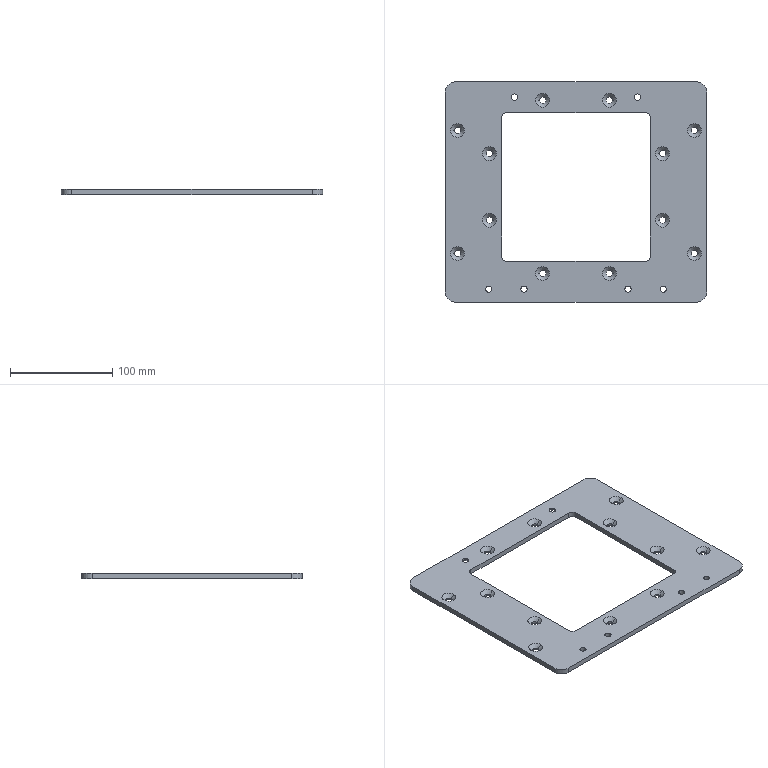NC program | NX | posted with a generic post | part box 255 x 215 x 5 mm
Lines 1056 to 1866 of 7663:
(PLANAR_MILL_COPY_COPY_COPY_COPY , TOOL : D6A45)
N2086 T01 M6
N2088 G54
N2090 G17 G0 G90 X60.866 Y93.85 S9500 M3
N2092 G43 Z30. H1
N2094 Z0.
N2096 G94 G1 Z-1.5 F1250.
N2098 G3 X60. Y94.35 R1.
N2100 X58.15 Y92.5 R1.85
N2102 X60. Y94.35 R-1.85
N2104 X59.134 Y93.85 R1.
N2106 G1 Z0.
N2108 G0 Z30.
N2110 X-59.134
N2112 Z0.
N2114 G1 Z-1.5
N2116 G3 X-60. Y94.35 R1.
N2118 X-61.85 Y92.5 R1.85
N2120 X-60. Y94.35 R-1.85
N2122 X-60.866 Y93.85 R1.
N2124 G1 Z0.
N2126 G0 Z30.
N2128 X0.866 Y75.6
N2130 Z0.
N2132 G1 Z-1.5
N2134 G3 X0. Y76.1 R1.
N2136 G1 X-67.5
N2138 G3 X-71.1 Y72.5 R3.6
N2140 G1 Y-62.5
N2142 G3 X-67.5 Y-66.1 R3.6
N2144 G1 X67.5
N2146 G3 X71.1 Y-62.5 R3.6
N2148 G1 Y72.5
N2150 G3 X67.5 Y76.1 R3.6
N2152 G1 X0.
N2154 G3 X-0.866 Y75.6 R1.
N2156 G1 Z0.
N2158 G0 Z30.
N2160 Y109.4
N2162 Z0.
N2164 G1 Z-1.5
N2166 G3 X0. Y108.9 R1.
N2168 G1 X117.5
N2170 G2 X128.9 Y97.5 R11.4
N2172 G1 Y-97.5
N2174 G2 X117.5 Y-108.9 R11.4
N2176 G1 X-117.5
N2178 G2 X-128.9 Y-97.5 R11.4
N2180 G1 Y97.5
N2182 G2 X-117.5 Y108.9 R11.4
N2184 G1 X0.
N2186 G3 X0.866 Y109.4 R1.
N2188 G1 Z0.
N2190 G0 Z30.
N2192 X-86.116 Y-95.95
N2194 Z0.
N2196 G1 Z-1.5
N2198 G3 X-85.25 Y-96.45 R1.
N2200 X-83.65 Y-94.85 R1.6
N2202 X-85.25 Y-96.45 R-1.6
N2204 X-84.384 Y-95.95 R1.
N2206 G1 Z0.
N2208 G0 Z30.
N2210 X-51.616
N2212 Z0.
N2214 G1 Z-1.5
N2216 G3 X-50.75 Y-96.45 R1.
N2218 X-49.15 Y-94.85 R1.6
N2220 X-50.75 Y-96.45 R-1.6
N2222 X-49.884 Y-95.95 R1.
N2224 G1 Z0.
N2226 G0 Z30.
N2228 X49.884
N2230 Z0.
N2232 G1 Z-1.5
N2234 G3 X50.75 Y-96.45 R1.
N2236 X52.35 Y-94.85 R1.6
N2238 X50.75 Y-96.45 R-1.6
N2240 X51.616 Y-95.95 R1.
N2242 G1 Z0.
N2244 G0 Z30.
N2246 X84.384
N2248 Z0.
N2250 G1 Z-1.5
N2252 G3 X85.25 Y-96.45 R1.
N2254 X86.85 Y-94.85 R1.6
N2256 X85.25 Y-96.45 R-1.6
N2258 X86.116 Y-95.95 R1.
N2260 G1 Z0.
N2262 G0 Z30.
(ZLEVEL_PROFILE_COPY_1_COPY_1 , TOOL : D6A45)
N2264 X90.234 Y-29.265
N2266 Z1.5
N2268 G1 X90.456 Y-28.391 Z1.453 F1000.
N2270 X90.493 Y-28.098 Z1.437
N2272 Y-26.897 Z1.374
N2274 X90.106 Y-25.296 Z1.288
N2276 X89.3 Y-23.86 Z1.202
N2278 X88.136 Y-22.696 Z1.115
N2280 X86.699 Y-21.891 Z1.029
N2282 X85.098 Y-21.505 Z0.943
N2284 X83.453 Y-21.568 Z0.856
N2286 X82.297 Y-21.894 Z0.794
N2288 X80.879 Y-22.687 Z0.708
N2290 X79.725 Y-23.831 Z0.623
N2292 X78.918 Y-25.241 Z0.538
N2294 X78.518 Y-26.816 Z0.453
N2296 X78.554 Y-28.441 Z0.368
N2298 X79.022 Y-29.996 Z0.283
N2300 X79.89 Y-31.37 Z0.197
N2302 X80.75 Y-32.208 Z0.135
N2304 X82.146 Y-33.04 Z0.049
N2306 X83.714 Y-33.468 Z-0.036
N2308 X85.339 Y-33.461 Z-0.121
N2310 X86.903 Y-33.02 Z-0.206
N2312 X88.292 Y-32.177 Z-0.291
N2314 X89.405 Y-30.993 Z-0.376
N2316 X90.161 Y-29.554 Z-0.462
N2318 X90.456 Y-28.391 Z-0.524
N2320 X90.493 Y-28.098 Z-0.54
N2322 Y-27.497 Z-0.571
N2324 G3 X84.501 Y-21.506 R5.992 F1500.
N2326 X90.493 Y-27.497 R-5.992
N2328 G1 X90.44 Y-26.948 Z-0.58
N2330 X90.382 Y-26.4 Z-0.589
N2332 X90.112 Y-25.492 Z-0.604
N2334 X90.061 Y-25.346 Z-0.607
N2336 X89.788 Y-24.792 Z-0.616
N2338 X89.556 Y-24.373 Z-0.624
N2340 X89.203 Y-23.898 Z-0.634
N2342 X88.883 Y-23.511 Z-0.642
N2344 X88.451 Y-23.11 Z-0.651
N2346 X88.066 Y-22.789 Z-0.659
N2348 X87.568 Y-22.473 Z-0.668
N2350 X87.133 Y-22.231 Z-0.676
N2352 X86.584 Y-22.011 Z-0.686
N2354 X86.117 Y-21.855 Z-0.694
N2356 X85.536 Y-21.738 Z-0.703
N2358 X85.052 Y-21.671 Z-0.711
N2360 X84.462 Y-21.663 Z-0.72
N2362 X83.975 Y-21.686 Z-0.728
N2364 X83.391 Y-21.787 Z-0.738
N2366 X82.922 Y-21.897 Z-0.745
N2368 X82.354 Y-22.11 Z-0.755
N2370 X81.898 Y-22.313 Z-0.763
N2372 X81.383 Y-22.627 Z-0.772
N2374 X80.974 Y-22.912 Z-0.78
N2376 X80.18 Y-23.671 Z-0.798
N2378 X80.106 Y-23.766 Z-0.8
N2380 X79.55 Y-24.568 Z-0.816
N2382 X79.307 Y-25.068 Z-0.824
N2384 X79.101 Y-25.563 Z-0.833
N2386 X78.943 Y-26.143 Z-0.843
N2388 X78.848 Y-26.623 Z-0.85
N2390 X78.798 Y-27.21 Z-0.86
N2392 X78.807 Y-27.707 Z-0.868
N2394 X78.848 Y-28.133 Z-0.874
N2396 X78.888 Y-28.492 Z-0.88
N2398 X78.966 Y-28.777 Z-0.885
N2400 X79.135 Y-29.289 Z-0.894
N2402 X79.324 Y-29.795 Z-0.902
N2404 X79.586 Y-30.297 Z-0.911
N2406 X79.867 Y-30.723 Z-0.919
N2408 X80.124 Y-31.049 Z-0.926
N2410 X80.348 Y-31.33 Z-0.932
N2412 X80.573 Y-31.529 Z-0.936
N2414 X80.986 Y-31.868 Z-0.945
N2416 X81.417 Y-32.185 Z-0.954
N2418 X81.746 Y-32.376 Z-0.96
N2420 X82.055 Y-32.553 Z-0.965
N2422 X82.366 Y-32.668 Z-0.971
N2424 X82.871 Y-32.832 Z-0.979
N2426 X83.387 Y-32.961 Z-0.988
N2428 X83.494 Y-32.979 Z-0.989
N2430 X83.966 Y-33.037 Z-0.997
N2432 X84.441 Y-33.056 Z-1.004
N2434 X85.051 Y-33.038 Z-1.014
N2436 X85.197 Y-33.01 Z-1.017
N2438 X85.491 Y-32.95 Z-1.021
N2440 X86.001 Y-32.822 Z-1.03
N2442 X86.499 Y-32.647 Z-1.038
N2444 X86.866 Y-32.491 Z-1.044
N2446 X87.049 Y-32.409 Z-1.048
N2448 X87.428 Y-32.162 Z-1.055
N2450 X87.855 Y-31.859 Z-1.063
N2452 X88.246 Y-31.511 Z-1.072
N2454 X88.538 Y-31.225 Z-1.078
N2456 X88.672 Y-31.071 Z-1.081
N2458 X88.924 Y-30.719 Z-1.088
N2460 X89.206 Y-30.283 Z-1.096
N2462 X89.438 Y-29.817 Z-1.105
N2464 X89.633 Y-29.336 Z-1.113
N2466 X89.772 Y-28.836 Z-1.121
N2468 X89.843 Y-28.506 Z-1.127
N2470 X89.887 Y-28.171 Z-1.132
N2472 X89.906 Y-27.834 Z-1.137
N2474 X89.917 Y-27.497 Z-1.143
N2476 X89.88 Y-27.034 Z-1.151
N2478 X89.843 Y-26.571 Z-1.159
N2480 X89.725 Y-26.16 Z-1.167
N2482 X89.584 Y-25.681 Z-1.176
N2484 X89.307 Y-25.106 Z-1.187
N2486 X89.086 Y-24.668 Z-1.196
N2488 X88.737 Y-24.23 Z-1.206
N2490 X88.378 Y-23.795 Z-1.216
N2492 X87.947 Y-23.429 Z-1.226
N2494 X87.507 Y-23.092 Z-1.235
N2496 X86.992 Y-22.799 Z-1.246
N2498 X86.516 Y-22.585 Z-1.255
N2500 X85.916 Y-22.379 Z-1.266
N2502 X85.447 Y-22.295 Z-1.275
N2504 X84.899 Y-22.229 Z-1.285
N2506 X84.345 Z-1.294
N2508 X83.858 Y-22.261 Z-1.303
N2510 X83.558 Y-22.327 Z-1.308
N2512 X83.257 Y-22.391 Z-1.314
N2514 X82.648 Y-22.606 Z-1.325
N2516 X82.228 Y-22.772 Z-1.333
N2518 X81.72 Y-23.09 Z-1.344
N2520 X81.301 Y-23.354 Z-1.353
N2522 X80.529 Y-24.126 Z-1.372
N2524 X80.23 Y-24.571 Z-1.382
N2526 X79.938 Y-25.037 Z-1.391
N2528 X79.715 Y-25.551 Z-1.401
N2530 X79.545 Y-26.044 Z-1.41
N2532 X79.407 Y-26.645 Z-1.421
N2534 X79.364 Y-27.106 Z-1.43
N2536 X79.38 Y-27.741 Z-1.441
N2538 X79.415 Y-28.179 Z-1.449
N2540 X79.552 Y-28.748 Z-1.459
N2542 X79.681 Y-29.216 Z-1.468
N2544 X80.151 Y-30.175 Z-1.486
N2546 X80.3 Y-30.363 Z-1.491
N2548 X80.445 Y-30.555 Z-1.495
N2550 X80.819 Y-31.004 Z-1.505
N2552 X81.24 Y-31.35 Z-1.515
N2554 X81.643 Y-31.671 Z-1.524
N2556 X82.115 Y-31.93 Z-1.534
N2558 X82.582 Y-32.152 Z-1.543
N2560 X83.111 Y-32.326 Z-1.553
N2562 X83.595 Y-32.429 Z-1.561
N2564 X84.15 Y-32.489 Z-1.571
N2566 X84.566 Y-32.495 Z-1.579
N2568 X85.127 Y-32.441 Z-1.589
N2570 X85.528 Y-32.372 Z-1.596
N2572 X86.049 Y-32.214 Z-1.605
N2574 X86.445 Y-32.066 Z-1.613
N2576 X86.912 Y-31.815 Z-1.622
N2578 X87.283 Y-31.591 Z-1.63
N2580 X87.68 Y-31.26 Z-1.639
N2582 X88.012 Y-30.964 Z-1.647
N2584 X88.325 Y-30.572 Z-1.656
N2586 X88.604 Y-30.211 Z-1.664
N2588 X88.826 Y-29.778 Z-1.672
N2590 X89.039 Y-29.361 Z-1.681
N2592 X89.304 Y-28.445 Z-1.698
N2594 X89.327 Y-27.972 Z-1.706
N2596 X89.349 Y-27.498 Z-1.714
N2598 X89.295 Y-26.856 Z-1.727
N2600 X89.221 Y-26.483 Z-1.735
N2602 X89.106 Y-26.091 Z-1.743
N2604 X89.006 Y-25.766 Z-1.749
N2606 X88.885 Y-25.523 Z-1.755
N2608 X88.633 Y-25.083 Z-1.765
N2610 X88.353 Y-24.661 Z-1.775
N2612 X88.123 Y-24.376 Z-1.782
N2614 X88.005 Y-24.236 Z-1.786
N2616 X87.657 Y-23.93 Z-1.795
N2618 X87.144 Y-23.55 Z-1.808
N2620 X86.829 Y-23.362 Z-1.815
N2622 X86.283 Y-23.117 Z-1.827
N2624 X85.904 Y-22.979 Z-1.835
N2626 X85.357 Y-22.868 Z-1.846
N2628 X84.922 Y-22.801 Z-1.855
N2630 X84.438 Y-22.808 Z-1.865
N2632 X83.928 Y-22.837 Z-1.875
N2634 X83.222 Y-22.992 Z-1.889
N2636 X82.98 Y-23.083 Z-1.894
N2638 X82.539 Y-23.289 Z-1.904
N2640 X82.107 Y-23.516 Z-1.914
N2642 X81.679 Y-23.804 Z-1.924
N2644 X81.565 Y-23.905 Z-1.927
N2646 X81.345 Y-24.115 Z-1.933
N2648 X80.922 Y-24.58 Z-1.946
N2650 X80.725 Y-24.856 Z-1.952
N2652 X80.43 Y-25.361 Z-1.964
N2654 X80.271 Y-25.704 Z-1.972
N2656 X80.093 Y-26.255 Z-1.983
N2658 X79.996 Y-26.624 Z-1.991
N2660 X79.944 Y-27.146 Z-2.001
N2662 X79.928 Y-27.579 Z-2.01
N2664 X79.992 Y-28.073 Z-2.02
N2666 X80.069 Y-28.522 Z-2.029
N2668 X80.228 Y-28.999 Z-2.039
N2670 X80.397 Y-29.412 Z-2.048
N2672 X80.635 Y-29.831 Z-2.057
N2674 X80.899 Y-30.212 Z-2.067
N2676 X81.365 Y-30.727 Z-2.081
N2678 X81.465 Y-30.802 Z-2.083
N2680 X81.551 Y-30.89 Z-2.085
N2682 X81.946 Y-31.174 Z-2.095
N2684 X82.327 Y-31.418 Z-2.104
N2686 X82.788 Y-31.61 Z-2.114
N2688 X83.193 Y-31.77 Z-2.123
N2690 X83.662 Y-31.855 Z-2.132
N2692 X84.111 Y-31.932 Z-2.141
N2694 X84.577 Y-31.919 Z-2.151
N2696 X85.038 Y-31.898 Z-2.16
N2698 X85.501 Y-31.793 Z-2.169
N2700 X85.935 Y-31.674 Z-2.178
N2702 X86.381 Y-31.477 Z-2.188
N2704 X86.763 Y-31.27 Z-2.197
N2706 X87.185 Y-30.98 Z-2.207
N2708 X87.486 Y-30.705 Z-2.215
N2710 X87.862 Y-30.289 Z-2.226
N2712 X88.074 Y-30.005 Z-2.233
N2714 X88.326 Y-29.574 Z-2.243
N2716 X88.501 Y-29.201 Z-2.251
N2718 X88.605 Y-28.878 Z-2.258
N2720 X88.706 Y-28.555 Z-2.265
N2722 X88.75 Y-28.365 Z-2.268
N2724 X88.794 Y-27.932 Z-2.277
N2726 X88.817 Y-27.498 Z-2.286
N2728 X88.813 Y-27.393 Z-2.288
N2730 X88.808 Y-27.289 Z-2.29
N2732 X88.753 Y-26.784 Z-2.302
N2734 X88.684 Y-26.513 Z-2.308
N2736 X88.559 Y-26.105 Z-2.317
N2738 X88.491 Y-25.903 Z-2.322
N2740 X88.325 Y-25.593 Z-2.33
N2742 X87.967 Y-25.018 Z-2.345
N2744 X87.777 Y-24.777 Z-2.352
N2746 X87.355 Y-24.359 Z-2.365
N2748 X87.059 Y-24.111 Z-2.374
N2750 X86.593 Y-23.825 Z-2.386
N2752 X86.208 Y-23.634 Z-2.396
N2754 X85.705 Y-23.453 Z-2.408
N2756 X85.564 Y-23.415 Z-2.411
N2758 X85.274 Y-23.369 Z-2.417
N2760 X84.609 Y-23.309 Z-2.432
N2762 X84.309 Y-23.317 Z-2.439
N2764 X83.725 Y-23.4 Z-2.452
N2766 X83.361 Y-23.485 Z-2.461
N2768 X82.925 Y-23.653 Z-2.471
N2770 X82.476 Y-23.871 Z-2.482
N2772 X82.358 Y-23.942 Z-2.485
N2774 X82.246 Y-24.022 Z-2.488
N2776 X81.956 Y-24.209 Z-2.496
N2778 X81.71 Y-24.453 Z-2.504
N2780 X81.254 Y-24.962 Z-2.519
N2782 X81.095 Y-25.187 Z-2.525
N2784 X80.817 Y-25.693 Z-2.538
N2786 X80.667 Y-26.039 Z-2.546
N2788 X80.521 Y-26.56 Z-2.559
N2790 X80.451 Y-26.965 Z-2.568
N2792 X80.42 Y-27.32 Z-2.576
N2794 X80.41 Y-27.497 Z-2.58
N2796 X80.457 Y-27.911 Z-2.589
N2798 X80.58 Y-28.521 Z-2.603
N2800 X80.675 Y-28.828 Z-2.61
N2802 X80.903 Y-29.323 Z-2.622
N2804 X81.099 Y-29.666 Z-2.631
N2806 X81.415 Y-30.078 Z-2.643
N2808 X81.704 Y-30.378 Z-2.652
N2810 X82.058 Y-30.682 Z-2.662
N2812 X82.454 Y-30.929 Z-2.673
N2814 X82.679 Y-31.055 Z-2.678
N2816 X83.046 Y-31.203 Z-2.687
N2818 X83.304 Y-31.298 Z-2.693
N2820 X83.817 Y-31.404 Z-2.705
N2822 X84.214 Y-31.454 Z-2.714
N2824 X84.717 Y-31.445 Z-2.725
N2826 X85.132 Y-31.393 Z-2.735
N2828 X85.469 Y-31.317 Z-2.742
N2830 X85.638 Y-31.277 Z-2.746
N2832 X86.006 Y-31.125 Z-2.755
N2834 X86.526 Y-30.847 Z-2.768
N2836 X86.795 Y-30.67 Z-2.775
N2838 X87.18 Y-30.328 Z-2.787
N2840 X87.451 Y-30.043 Z-2.796
N2842 X87.744 Y-29.637 Z-2.807
N2844 X87.941 Y-29.285 Z-2.816
N2846 X88.13 Y-28.866 Z-2.826
N2848 X88.17 Y-28.725 Z-2.829
N2850 X88.243 Y-28.439 Z-2.836
N2852 X88.286 Y-28.206 Z-2.841
N2854 X88.322 Y-27.971 Z-2.847
N2856 X88.342 Y-27.498 Z-2.857
N2858 X88.336 Y-27.382 Z-2.86
N2860 X88.329 Y-27.267 Z-2.863
N2862 X88.29 Y-26.92 Z-2.872
N2864 X88.261 Y-26.748 Z-2.876
N2866 X88.229 Y-26.645 Z-2.879
N2868 X88.165 Y-26.438 Z-2.885
N2870 X88.045 Y-26.074 Z-2.894
N2872 X87.907 Y-25.813 Z-2.902
N2874 X87.803 Y-25.631 Z-2.907
N2876 X87.463 Y-25.144 Z-2.922
N2878 X87.274 Y-24.927 Z-2.929
N2880 X86.988 Y-24.666 Z-2.939
N2882 X86.588 Y-24.38 Z-2.952
N2884 X86.353 Y-24.243 Z-2.959
N2886 X86.086 Y-24.106 Z-2.966
N2888 X85.805 Y-24.001 Z-2.974
N2890 X85.274 Y-23.848 Z-2.988
N2892 X84.961 Y-23.801 Z-2.996
N2894 X84.579 Y-23.756 Z-3.006
N2896 X84.29 Y-23.769 Z-3.013
N2898 X84.094 Y-23.79 Z-3.018
N2900 X83.568 Y-23.9 Z-3.031
N2902 X83.256 Y-24.005 Z-3.04
N2904 X82.794 Y-24.22 Z-3.053
N2906 X82.494 Y-24.404 Z-3.061
N2908 X82.1 Y-24.715 Z-3.074
N2910 X81.85 Y-24.966 Z-3.083
N2912 X81.541 Y-25.356 Z-3.096
N2914 X81.355 Y-25.656 Z-3.105
N2916 X81.146 Y-26.105 Z-3.117
N2918 X81.035 Y-26.437 Z-3.126
N2920 X80.935 Y-26.919 Z-3.138
N2922 X80.905 Y-27.266 Z-3.147
N2924 X80.919 Y-27.755 Z-3.16
N2926 X80.968 Y-28.097 Z-3.168
N2928 X81.094 Y-28.567 Z-3.181
N2930 X81.22 Y-28.887 Z-3.189
N2932 X81.449 Y-29.312 Z-3.202
N2934 X81.645 Y-29.593 Z-3.21
N2936 X81.964 Y-29.952 Z-3.222
N2938 X82.217 Y-30.178 Z-3.231
N2940 X82.606 Y-30.451 Z-3.243
N2942 X82.905 Y-30.614 Z-3.252
N2944 X83.333 Y-30.786 Z-3.263
N2946 X83.652 Y-30.873 Z-3.272
N2948 X84.107 Y-30.944 Z-3.283
N2950 X84.433 Y-30.958 Z-3.292
N2952 X84.89 Y-30.925 Z-3.303
N2954 X85.209 Y-30.865 Z-3.312
N2956 X85.645 Y-30.73 Z-3.323
N2958 X85.94 Y-30.601 Z-3.331
N2960 X86.332 Y-30.373 Z-3.343
N2962 X86.589 Y-30.181 Z-3.351
N2964 X86.872 Y-29.921 Z-3.361
N2966 X87.124 Y-29.629 Z-3.371
N2968 X87.198 Y-29.529 Z-3.374
N2970 X87.269 Y-29.427 Z-3.377
N2972 X87.403 Y-29.206 Z-3.383
N2974 X87.519 Y-28.975 Z-3.39
N2976 X87.68 Y-28.548 Z-3.402
N2978 X87.755 Y-28.252 Z-3.409
N2980 X87.81 Y-27.878 Z-3.419
N2982 X87.821 Y-27.499 Z-3.429
N2984 X87.817 Y-27.398 Z-3.432
N2986 X87.809 Y-27.299 Z-3.435
N2988 X87.72 Y-26.781 Z-3.45
N2990 X87.635 Y-26.5 Z-3.459
N2992 X87.44 Y-26.055 Z-3.474
N2994 X87.272 Y-25.773 Z-3.484
N2996 X86.983 Y-25.4 Z-3.498
N2998 X86.745 Y-25.163 Z-3.508
N3000 X86.371 Y-24.872 Z-3.522
N3002 X86.09 Y-24.705 Z-3.532
N3004 X85.649 Y-24.522 Z-3.546
N3006 X85.33 Y-24.419 Z-3.556
N3008 X84.892 Y-24.353 Z-3.57
N3010 X84.53 Y-24.334 Z-3.581
N3012 X84.085 Y-24.38 Z-3.594
N3014 X83.74 Y-24.453 Z-3.605
N3016 X83.322 Y-24.615 Z-3.618
N3018 X83.011 Y-24.763 Z-3.629
N3020 X82.657 Y-25.005 Z-3.642
N3022 X82.388 Y-25.243 Z-3.653
N3024 X82.101 Y-25.585 Z-3.666
N3026 X81.91 Y-25.859 Z-3.676
N3028 X81.721 Y-26.253 Z-3.689
N3030 X81.603 Y-26.57 Z-3.699
N3032 X81.538 Y-26.829 Z-3.707
N3034 X81.514 Y-26.961 Z-3.712
N3036 X81.505 Y-27.083 Z-3.715
N3038 X81.49 Y-27.329 Z-3.723
N3040 X81.513 Y-27.74 Z-3.735
N3042 X81.542 Y-27.992 Z-3.743
N3044 X81.631 Y-28.345 Z-3.754
N3046 X81.741 Y-28.623 Z-3.763
N3048 X81.895 Y-28.92 Z-3.773
N3050 X82.079 Y-29.185 Z-3.783
N3052 X82.43 Y-29.592 Z-3.799
N3054 X82.559 Y-29.705 Z-3.804
N3056 X82.917 Y-29.959 Z-3.817
N3058 X83.15 Y-30.085 Z-3.825
N3060 X83.523 Y-30.223 Z-3.837
N3062 X83.811 Y-30.308 Z-3.846
N3064 X84.199 Y-30.364 Z-3.858
N3066 X84.501 Y-30.375 Z-3.867
N3068 X84.88 Y-30.334 Z-3.879
N3070 X85.181 Y-30.271 Z-3.888
N3072 X85.546 Y-30.127 Z-3.9
N3074 X85.813 Y-30.013 Z-3.909
N3076 X86.105 Y-29.818 Z-3.919
N3078 X86.359 Y-29.61 Z-3.929
N3080 X86.597 Y-29.361 Z-3.939
N3082 X86.785 Y-29.09 Z-3.949
N3084 X86.917 Y-28.842 Z-3.958
N3086 X87.046 Y-28.592 Z-3.966
N3088 X87.173 Y-28.207 Z-3.979
N3090 X87.204 Y-28.055 Z-3.983
N3092 X87.243 Y-27.499 Z-4.
N3094 G3 X84.501 Y-24.763 R2.739
N3096 X87.243 Y-27.499 R-2.739
N3098 G1 Z-2.5
N3100 G0 Z30.
N3102 X121.245 Y-61.728
N3104 Z1.5
N3106 G1 X121.496 Y-60.602 Z1.44 F1000.
N3108 Y-59.401 Z1.377
N3110 X121.168 Y-57.955 Z1.299
N3112 X120.498 Y-56.633 Z1.221
N3114 X119.525 Y-55.515 Z1.144
N3116 X118.555 Y-54.806 Z1.081
N3118 X117.055 Y-54.178 Z0.995
N3120 X115.441 Y-53.974 Z0.91
N3122 X113.831 Y-54.209 Z0.825
N3124 X112.343 Y-54.865 Z0.74
N3126 X111.085 Y-55.896 Z0.654
N3128 X110.148 Y-57.226 Z0.569
N3130 X109.6 Y-58.757 Z0.484
N3132 X109.471 Y-59.952 Z0.421
N3134 X109.677 Y-61.565 Z0.336
N3136 X110.307 Y-63.065 Z0.25
N3138 X111.315 Y-64.341 Z0.165
N3140 X112.628 Y-65.302 Z0.08
N3142 X114.15 Y-65.876 Z-0.005
N3144 X115.77 Y-66.023 Z-0.091
N3146 X117.37 Y-65.731 Z-0.176
N3148 X118.469 Y-65.246 Z-0.239
N3150 X119.626 Y-64.394 Z-0.314
N3152 X120.548 Y-63.293 Z-0.389
N3154 X121.184 Y-62.004 Z-0.465
N3156 X121.496 Y-60.602 Z-0.54
N3158 Y-60.001 Z-0.571
N3160 G3 X115.498 Y-54.003 R5.998 F1500.
N3162 X121.496 Y-60.001 R-5.998
N3164 G1 X121.446 Y-59.442 Z-0.58
N3166 X121.373 Y-58.885 Z-0.589
N3168 X121.22 Y-58.313 Z-0.599
N3170 X121.044 Y-57.814 Z-0.607
N3172 X120.77 Y-57.249 Z-0.617
N3174 X120.523 Y-56.826 Z-0.625
N3176 X120.147 Y-56.322 Z-0.635
N3178 X119.829 Y-55.956 Z-0.643
N3180 X119.366 Y-55.531 Z-0.653
N3182 X118.987 Y-55.233 Z-0.661
N3184 X118.447 Y-54.898 Z-0.671
N3186 X118.014 Y-54.675 Z-0.678
N3188 X117.487 Y-54.489 Z-0.687
N3190 X116.956 Y-54.313 Z-0.696
N3192 X116.546 Y-54.236 Z-0.703
N3194 X116.2 Y-54.192 Z-0.708
N3196 X115.852 Y-54.158 Z-0.714
N3198 X115.227 Y-54.164 Z-0.724
N3200 X114.742 Y-54.215 Z-0.732
N3202 X114.323 Y-54.3 Z-0.739
N3204 X113.959 Y-54.371 Z-0.745
N3206 X113.667 Y-54.481 Z-0.75
N3208 X113.161 Y-54.701 Z-0.758
N3210 X112.665 Y-54.944 Z-0.767
N3212 X112.338 Y-55.154 Z-0.773
N3214 X112.027 Y-55.351 Z-0.779
N3216 X111.771 Y-55.586 Z-0.785
N3218 X111.382 Y-55.973 Z-0.793
N3220 X111.017 Y-56.383 Z-0.802
N3222 X110.668 Y-56.862 Z-0.812
N3224 X110.578 Y-57.003 Z-0.814
N3226 X110.429 Y-57.305 Z-0.82
N3228 X110.209 Y-57.803 Z-0.828
N3230 X110.027 Y-58.318 Z-0.837
N3232 X109.87 Y-58.911 Z-0.847
N3234 X109.851 Y-59.069 Z-0.849
N3236 X109.822 Y-59.385 Z-0.855
N3238 X109.797 Y-59.927 Z-0.863
N3240 X109.824 Y-60.47 Z-0.872
N3242 X109.903 Y-61.004 Z-0.88
N3244 X110.035 Y-61.529 Z-0.889
N3246 X110.16 Y-61.913 Z-0.896
N3248 X110.44 Y-62.527 Z-0.906
N3250 X110.623 Y-62.888 Z-0.913
N3252 X110.836 Y-63.176 Z-0.918
N3254 X111.023 Y-63.428 Z-0.923
N3256 X111.451 Y-63.912 Z-0.934
N3258 X111.764 Y-64.201 Z-0.941
N3260 X112.269 Y-64.589 Z-0.951
N3262 X112.635 Y-64.817 Z-0.958
N3264 X113.197 Y-65.098 Z-0.968
N3266 X113.603 Y-65.257 Z-0.975
N3268 X114.2 Y-65.423 Z-0.985
N3270 X114.635 Y-65.505 Z-0.992
N3272 X115.242 Y-65.553 Z-1.001
N3274 X115.691 Z-1.008
N3276 X116.286 Y-65.486 Z-1.018
N3278 X116.735 Y-65.4 Z-1.025
N3280 X117.304 Y-65.222 Z-1.035
N3282 X117.728 Y-65.053 Z-1.042
N3284 X118.254 Y-64.769 Z-1.052
N3286 X118.644 Y-64.519 Z-1.059
N3288 X119.045 Y-64.176 Z-1.067
N3290 X119.438 Y-63.822 Z-1.076
N3292 X119.561 Y-63.685 Z-1.079
N3294 X119.682 Y-63.545 Z-1.082
N3296 X120.083 Y-62.989 Z-1.093
N3298 X120.356 Y-62.487 Z-1.102
N3300 X120.554 Y-62.05 Z-1.109
N3302 X120.734 Y-61.481 Z-1.119
N3304 X120.84 Y-61.042 Z-1.126
N3306 X120.888 Y-60.522 Z-1.135
N3308 X120.921 Y-60.001 Z-1.143
N3310 X120.869 Y-59.274 Z-1.156
N3312 X120.809 Y-58.93 Z-1.162
N3314 X120.635 Y-58.346 Z-1.173
N3316 X120.47 Y-57.913 Z-1.181
N3318 X120.212 Y-57.446 Z-1.19
N3320 X119.941 Y-56.986 Z-1.2
N3322 X119.777 Y-56.769 Z-1.205
N3324 X119.52 Y-56.467 Z-1.212
N3326 X119.244 Y-56.183 Z-1.219
N3328 X118.781 Y-55.773 Z-1.23
N3330 X118.406 Y-55.535 Z-1.238
N3332 X117.946 Y-55.276 Z-1.247
N3334 X117.461 Y-55.067 Z-1.256
N3336 X117.075 Y-54.928 Z-1.263
N3338 X116.877 Y-54.88 Z-1.267
N3340 X116.445 Y-54.794 Z-1.275
N3342 X115.78 Y-54.732 Z-1.287
N3344 X115.343 Y-54.727 Z-1.295
N3346 X114.723 Y-54.804 Z-1.306
N3348 X114.253 Y-54.887 Z-1.314
N3350 X113.68 Y-55.095 Z-1.325
N3352 X113.221 Y-55.266 Z-1.334
N3354 X112.765 Y-55.561 Z-1.343
N3356 X112.301 Y-55.862 Z-1.353
N3358 X111.914 Y-56.239 Z-1.362
N3360 X111.531 Y-56.635 Z-1.372
N3362 X111.283 Y-56.992 Z-1.38
N3364 X110.939 Y-57.545 Z-1.391
N3366 X110.838 Y-57.761 Z-1.396
N3368 X110.732 Y-57.975 Z-1.4
N3370 X110.548 Y-58.552 Z-1.411
N3372 X110.45 Y-58.962 Z-1.418
N3374 X110.416 Y-59.169 Z-1.422
N3376 X110.37 Y-59.615 Z-1.43
N3378 X110.378 Y-60.271 Z-1.441
N3380 X110.407 Y-60.689 Z-1.449
N3382 X110.675 Y-61.728 Z-1.468
N3384 X111.16 Y-62.681 Z-1.487
N3386 X111.489 Y-63.089 Z-1.496
N3388 X111.831 Y-63.506 Z-1.506
N3390 X112.238 Y-63.854 Z-1.515
N3392 X112.654 Y-64.172 Z-1.524
N3394 X113.144 Y-64.454 Z-1.534
N3396 X113.592 Y-64.654 Z-1.543
N3398 X114.169 Y-64.837 Z-1.554
N3400 X114.604 Y-64.932 Z-1.562
N3402 X115.126 Y-64.968 Z-1.571
N3404 X115.649 Y-64.996 Z-1.58
N3406 X116.108 Y-64.957 Z-1.588
N3408 X116.682 Y-64.845 Z-1.599
N3410 X117.66 Y-64.485 Z-1.617
N3412 X118.532 Y-63.921 Z-1.635
N3414 X119.261 Y-63.188 Z-1.654
N3416 X119.75 Y-62.475 Z-1.669
N3418 X120.107 Y-61.69 Z-1.684
N3420 X120.323 Y-60.857 Z-1.699
N3422 X120.346 Y-60.001 Z-1.714
N3424 X120.326 Y-59.556 Z-1.723
N3426 X120.29 Y-59.208 Z-1.73
N3428 X120.215 Y-58.964 Z-1.735
N3430 X120.06 Y-58.47 Z-1.745
N3432 X119.866 Y-57.989 Z-1.756
N3434 X119.705 Y-57.678 Z-1.763
N3436 X119.624 Y-57.522 Z-1.766
N3438 X119.318 Y-57.116 Z-1.776
N3440 X119.082 Y-56.837 Z-1.783
N3442 X118.824 Y-56.578 Z-1.791
N3444 X118.624 Y-56.398 Z-1.796
N3446 X118.133 Y-56.047 Z-1.808
N3448 X117.8 Y-55.84 Z-1.816
N3450 X117.298 Y-55.624 Z-1.827
N3452 X116.88 Y-55.469 Z-1.836
N3454 X116.355 Y-55.367 Z-1.846
N3456 X115.907 Y-55.299 Z-1.855
N3458 X115.4 Y-55.307 Z-1.865
N3460 X114.925 Y-55.343 Z-1.875
N3462 X114.407 Y-55.45 Z-1.885
N3464 X113.978 Y-55.587 Z-1.894
N3466 X113.451 Y-55.802 Z-1.906
N3468 X113.106 Y-56.018 Z-1.914
N3470 X112.709 Y-56.297 Z-1.923
N3472 X112.344 Y-56.616 Z-1.933
N3474 X111.968 Y-57.023 Z-1.944
N3476 X111.722 Y-57.355 Z-1.952
N3478 X111.448 Y-57.831 Z-1.963
N3480 X111.268 Y-58.203 Z-1.972
N3482 X111.056 Y-58.892 Z-1.986
N3484 X110.995 Y-59.123 Z-1.991
N3486 X110.952 Y-59.634 Z-2.001
N3488 X110.928 Y-60.078 Z-2.01
N3490 X110.979 Y-60.559 Z-2.019
N3492 X111.069 Y-61.021 Z-2.029
N3494 X111.227 Y-61.525 Z-2.039
N3496 X111.397 Y-61.91 Z-2.048
N3498 X111.678 Y-62.395 Z-2.059
N3500 X111.897 Y-62.712 Z-2.067
N3502 X112.259 Y-63.105 Z-2.077
N3504 X112.549 Y-63.391 Z-2.085
N3506 X112.966 Y-63.68 Z-2.095
N3508 X113.324 Y-63.921 Z-2.104
N3510 X114.191 Y-64.274 Z-2.123
N3512 X115.111 Y-64.436 Z-2.141
N3514 X116.04 Y-64.403 Z-2.16
N3516 X116.377 Y-64.326 Z-2.167
N3518 X116.715 Y-64.254 Z-2.174
N3520 X116.819 Y-64.212 Z-2.176
N3522 X116.927 Y-64.18 Z-2.178
N3524 X117.394 Y-63.979 Z-2.188
N3526 X117.746 Y-63.783 Z-2.196
N3528 X118.177 Y-63.479 Z-2.207
N3530 X118.465 Y-63.229 Z-2.214
N3532 X118.822 Y-62.835 Z-2.225
N3534 X119.054 Y-62.542 Z-2.232
N3536 X119.299 Y-62.119 Z-2.242
N3538 X119.485 Y-61.751 Z-2.25
N3540 X119.639 Y-61.281 Z-2.26
N3542 X119.745 Y-60.892 Z-2.268
N3544 X119.784 Y-60.447 Z-2.277
N3546 X119.817 Y-60.001 Z-2.286
N3548 X119.801 Y-59.642 Z-2.294
N3550 X119.772 Y-59.355 Z-2.3
N3552 X119.714 Y-59.144 Z-2.305
N3554 X119.588 Y-58.735 Z-2.315
N3556 X119.445 Y-58.331 Z-2.324
N3558 X119.272 Y-57.984 Z-2.333
N3560 X119.021 Y-57.591 Z-2.343
N3562 X118.741 Y-57.239 Z-2.353
N3564 X118.46 Y-56.952 Z-2.362
N3566 X118.168 Y-56.687 Z-2.371
N3568 X118.008 Y-56.573 Z-2.375
N3570 X117.668 Y-56.367 Z-2.384
N3572 X117.118 Y-56.104 Z-2.398
N3574 X116.765 Y-55.982 Z-2.406
N3576 X116.391 Y-55.89 Z-2.415
N3578 X116.07 Y-55.833 Z-2.422
N3580 X115.802 Y-55.817 Z-2.428
N3582 X115.374 Y-55.813 Z-2.438
N3584 X115.16 Y-55.814 Z-2.442
N3586 X115.05 Y-55.835 Z-2.445
N3588 X114.831 Y-55.879 Z-2.45
N3590 X114.382 Y-55.967 Z-2.46
N3592 X114.083 Y-56.088 Z-2.467
N3594 X113.904 Y-56.162 Z-2.472
N3596 X113.367 Y-56.445 Z-2.485
N3598 X113.07 Y-56.648 Z-2.493
N3600 X112.781 Y-56.887 Z-2.502
N3602 X112.547 Y-57.107 Z-2.509
N3604 X112.376 Y-57.312 Z-2.515
N3606 X112.098 Y-57.701 Z-2.525
N3608 X111.855 Y-58.114 Z-2.536
N3610 X111.736 Y-58.361 Z-2.542
N3612 X111.646 Y-58.62 Z-2.548
N3614 X111.585 Y-58.814 Z-2.553
N3616 X111.535 Y-59.011 Z-2.557
N3618 X111.442 Y-59.622 Z-2.571
N3620 X111.426 Y-59.953 Z-2.579
N3622 X111.44 Y-60.309 Z-2.587
N3624 X111.473 Y-60.622 Z-2.594
N3626 X111.547 Y-60.889 Z-2.6
N3628 X111.67 Y-61.338 Z-2.61
N3630 X111.763 Y-61.549 Z-2.615
N3632 X111.875 Y-61.769 Z-2.621
N3634 X112.192 Y-62.291 Z-2.634
N3636 X112.394 Y-62.547 Z-2.642
N3638 X112.792 Y-62.953 Z-2.654
N3640 X113.073 Y-63.183 Z-2.663
N3642 X113.369 Y-63.376 Z-2.67
N3644 X113.633 Y-63.537 Z-2.677
N3646 X113.88 Y-63.639 Z-2.683
N3648 X114.277 Y-63.791 Z-2.693
N3650 X114.481 Y-63.845 Z-2.697
N3652 X114.765 Y-63.898 Z-2.704
N3654 X115.301 Y-63.953 Z-2.716
N3656 X115.682 Y-63.946 Z-2.724
N3658 X115.949 Y-63.914 Z-2.73
N3660 X116.216 Y-63.874 Z-2.737
N3662 X116.581 Y-63.783 Z-2.745
N3664 X117.035 Y-63.612 Z-2.756
N3666 X117.357 Y-63.451 Z-2.764
N3668 X117.634 Y-63.277 Z-2.771
N3670 X117.772 Y-63.189 Z-2.775
N3672 X117.868 Y-63.122 Z-2.777
N3674 X118.041 Y-62.963 Z-2.783
N3676 X118.339 Y-62.668 Z-2.792
N3678 X118.603 Y-62.341 Z-2.801
N3680 X118.866 Y-61.934 Z-2.812
N3682 X119.019 Y-61.618 Z-2.82
N3684 X119.186 Y-61.149 Z-2.831
N3686 X119.271 Y-60.826 Z-2.839
N3688 X119.314 Y-60.414 Z-2.848
N3690 X119.347 Y-60.001 Z-2.857
N3692 X119.32 Y-59.629 Z-2.867
N3694 X119.3 Y-59.443 Z-2.871